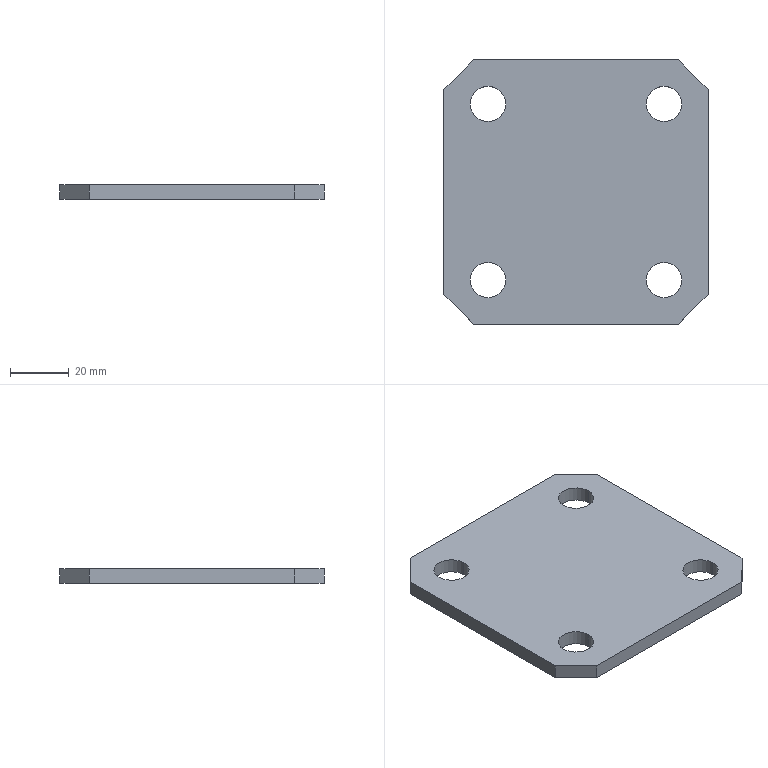Part | STEP file | Floating adjusting plate | 1 solid | 18 faces | box 90 x 90 x 5 mm | volume 37238 mm3 | plane 10 | cylinder 8 | commonest cylinder face diameters 12 x8
STEP:
#1=CARTESIAN_POINT('',(-24.,-30.,5.));
#2=VERTEX_POINT('',#1);
#3=CARTESIAN_POINT('',(-36.,-30.,5.));
#4=VERTEX_POINT('',#3);
#5=CARTESIAN_POINT('',(-30.,-30.,5.));
#6=DIRECTION('',(0.,0.,-1.));
#7=DIRECTION('',(1.,0.,0.));
#8=AXIS2_PLACEMENT_3D('',#5,#6,#7);
#9=CIRCLE('',#8,6.);
#10=EDGE_CURVE('',#2,#4,#9,.T.);
#11=ORIENTED_EDGE('',*,*,#10,.F.);
#12=CARTESIAN_POINT('',(-24.,-30.,0.));
#13=VERTEX_POINT('',#12);
#14=CARTESIAN_POINT('',(-24.,-30.,10.));
#15=DIRECTION('',(0.,0.,-1.));
#16=VECTOR('',#15,1000.);
#17=LINE('',#14,#16);
#18=EDGE_CURVE('',#2,#13,#17,.T.);
#19=ORIENTED_EDGE('',*,*,#18,.T.);
#20=CARTESIAN_POINT('',(-36.,-30.,0.));
#21=VERTEX_POINT('',#20);
#22=CARTESIAN_POINT('',(-30.,-30.,0.));
#23=DIRECTION('',(0.,0.,1.));
#24=DIRECTION('',(1.,0.,0.));
#25=AXIS2_PLACEMENT_3D('',#22,#23,#24);
#26=CIRCLE('',#25,6.);
#27=EDGE_CURVE('',#21,#13,#26,.T.);
#28=ORIENTED_EDGE('',*,*,#27,.F.);
#29=CARTESIAN_POINT('',(-36.,-30.,10.));
#30=DIRECTION('',(0.,0.,-1.));
#31=VECTOR('',#30,1000.);
#32=LINE('',#29,#31);
#33=EDGE_CURVE('',#4,#21,#32,.T.);
#34=ORIENTED_EDGE('',*,*,#33,.F.);
#35=EDGE_LOOP('',(#11,#19,#28,#34));
#36=FACE_OUTER_BOUND('',#35,.T.);
#37=CARTESIAN_POINT('',(-30.,-30.,10.));
#38=DIRECTION('',(0.,0.,-1.));
#39=DIRECTION('',(-1.,0.,0.));
#40=AXIS2_PLACEMENT_3D('',#37,#38,#39);
#41=CYLINDRICAL_SURFACE('',#40,6.);
#42=ADVANCED_FACE('',(#36),#41,.F.);
#43=CARTESIAN_POINT('',(-36.,30.,5.));
#44=VERTEX_POINT('',#43);
#45=CARTESIAN_POINT('',(-24.,30.,5.));
#46=VERTEX_POINT('',#45);
#47=CARTESIAN_POINT('',(-30.,30.,5.));
#48=DIRECTION('',(0.,0.,1.));
#49=DIRECTION('',(1.,0.,0.));
#50=AXIS2_PLACEMENT_3D('',#47,#48,#49);
#51=CIRCLE('',#50,6.);
#52=EDGE_CURVE('',#44,#46,#51,.T.);
#53=ORIENTED_EDGE('',*,*,#52,.T.);
#54=CARTESIAN_POINT('',(-24.,30.,0.));
#55=VERTEX_POINT('',#54);
#56=CARTESIAN_POINT('',(-24.,30.,10.));
#57=DIRECTION('',(0.,0.,-1.));
#58=VECTOR('',#57,1000.);
#59=LINE('',#56,#58);
#60=EDGE_CURVE('',#46,#55,#59,.T.);
#61=ORIENTED_EDGE('',*,*,#60,.T.);
#62=CARTESIAN_POINT('',(-36.,30.,0.));
#63=VERTEX_POINT('',#62);
#64=CARTESIAN_POINT('',(-30.,30.,0.));
#65=DIRECTION('',(0.,0.,-1.));
#66=DIRECTION('',(1.,0.,0.));
#67=AXIS2_PLACEMENT_3D('',#64,#65,#66);
#68=CIRCLE('',#67,6.);
#69=EDGE_CURVE('',#55,#63,#68,.T.);
#70=ORIENTED_EDGE('',*,*,#69,.T.);
#71=CARTESIAN_POINT('',(-36.,30.,10.));
#72=DIRECTION('',(0.,0.,-1.));
#73=VECTOR('',#72,1000.);
#74=LINE('',#71,#73);
#75=EDGE_CURVE('',#44,#63,#74,.T.);
#76=ORIENTED_EDGE('',*,*,#75,.F.);
#77=EDGE_LOOP('',(#53,#61,#70,#76));
#78=FACE_OUTER_BOUND('',#77,.T.);
#79=CARTESIAN_POINT('',(-30.,30.,10.));
#80=DIRECTION('',(0.,0.,-1.));
#81=DIRECTION('',(-1.,0.,0.));
#82=AXIS2_PLACEMENT_3D('',#79,#80,#81);
#83=CYLINDRICAL_SURFACE('',#82,6.);
#84=ADVANCED_FACE('',(#78),#83,.F.);
#85=CARTESIAN_POINT('',(36.,30.,5.));
#86=VERTEX_POINT('',#85);
#87=CARTESIAN_POINT('',(24.,30.,5.));
#88=VERTEX_POINT('',#87);
#89=CARTESIAN_POINT('',(30.,30.,5.));
#90=DIRECTION('',(0.,0.,-1.));
#91=DIRECTION('',(1.,0.,0.));
#92=AXIS2_PLACEMENT_3D('',#89,#90,#91);
#93=CIRCLE('',#92,6.);
#94=EDGE_CURVE('',#86,#88,#93,.T.);
#95=ORIENTED_EDGE('',*,*,#94,.F.);
#96=CARTESIAN_POINT('',(36.,30.,0.));
#97=VERTEX_POINT('',#96);
#98=CARTESIAN_POINT('',(36.,30.,10.));
#99=DIRECTION('',(0.,0.,-1.));
#100=VECTOR('',#99,1000.);
#101=LINE('',#98,#100);
#102=EDGE_CURVE('',#86,#97,#101,.T.);
#103=ORIENTED_EDGE('',*,*,#102,.T.);
#104=CARTESIAN_POINT('',(24.,30.,0.));
#105=VERTEX_POINT('',#104);
#106=CARTESIAN_POINT('',(30.,30.,0.));
#107=DIRECTION('',(0.,0.,1.));
#108=DIRECTION('',(-1.,0.,0.));
#109=AXIS2_PLACEMENT_3D('',#106,#107,#108);
#110=CIRCLE('',#109,6.);
#111=EDGE_CURVE('',#105,#97,#110,.T.);
#112=ORIENTED_EDGE('',*,*,#111,.F.);
#113=CARTESIAN_POINT('',(24.,30.,10.));
#114=DIRECTION('',(0.,0.,-1.));
#115=VECTOR('',#114,1000.);
#116=LINE('',#113,#115);
#117=EDGE_CURVE('',#88,#105,#116,.T.);
#118=ORIENTED_EDGE('',*,*,#117,.F.);
#119=EDGE_LOOP('',(#95,#103,#112,#118));
#120=FACE_OUTER_BOUND('',#119,.T.);
#121=CARTESIAN_POINT('',(30.,30.,10.));
#122=DIRECTION('',(0.,0.,-1.));
#123=DIRECTION('',(-1.,0.,0.));
#124=AXIS2_PLACEMENT_3D('',#121,#122,#123);
#125=CYLINDRICAL_SURFACE('',#124,6.);
#126=ADVANCED_FACE('',(#120),#125,.F.);
#127=CARTESIAN_POINT('',(24.,-30.,5.));
#128=VERTEX_POINT('',#127);
#129=CARTESIAN_POINT('',(36.,-30.,5.));
#130=VERTEX_POINT('',#129);
#131=CARTESIAN_POINT('',(30.,-30.,5.));
#132=DIRECTION('',(0.,0.,1.));
#133=DIRECTION('',(1.,0.,0.));
#134=AXIS2_PLACEMENT_3D('',#131,#132,#133);
#135=CIRCLE('',#134,6.);
#136=EDGE_CURVE('',#128,#130,#135,.T.);
#137=ORIENTED_EDGE('',*,*,#136,.T.);
#138=CARTESIAN_POINT('',(36.,-30.,0.));
#139=VERTEX_POINT('',#138);
#140=CARTESIAN_POINT('',(36.,-30.,10.));
#141=DIRECTION('',(0.,0.,-1.));
#142=VECTOR('',#141,1000.);
#143=LINE('',#140,#142);
#144=EDGE_CURVE('',#130,#139,#143,.T.);
#145=ORIENTED_EDGE('',*,*,#144,.T.);
#146=CARTESIAN_POINT('',(24.,-30.,0.));
#147=VERTEX_POINT('',#146);
#148=CARTESIAN_POINT('',(30.,-30.,0.));
#149=DIRECTION('',(0.,0.,-1.));
#150=DIRECTION('',(-1.,0.,0.));
#151=AXIS2_PLACEMENT_3D('',#148,#149,#150);
#152=CIRCLE('',#151,6.);
#153=EDGE_CURVE('',#139,#147,#152,.T.);
#154=ORIENTED_EDGE('',*,*,#153,.T.);
#155=CARTESIAN_POINT('',(24.,-30.,10.));
#156=DIRECTION('',(0.,0.,-1.));
#157=VECTOR('',#156,1000.);
#158=LINE('',#155,#157);
#159=EDGE_CURVE('',#128,#147,#158,.T.);
#160=ORIENTED_EDGE('',*,*,#159,.F.);
#161=EDGE_LOOP('',(#137,#145,#154,#160));
#162=FACE_OUTER_BOUND('',#161,.T.);
#163=CARTESIAN_POINT('',(30.,-30.,10.));
#164=DIRECTION('',(0.,0.,-1.));
#165=DIRECTION('',(-1.,0.,0.));
#166=AXIS2_PLACEMENT_3D('',#163,#164,#165);
#167=CYLINDRICAL_SURFACE('',#166,6.);
#168=ADVANCED_FACE('',(#162),#167,.F.);
#169=CARTESIAN_POINT('',(45.,-35.,0.));
#170=VERTEX_POINT('',#169);
#171=CARTESIAN_POINT('',(45.,35.,0.));
#172=VERTEX_POINT('',#171);
#173=CARTESIAN_POINT('',(45.,45.,0.));
#174=DIRECTION('',(0.,1.,0.));
#175=VECTOR('',#174,1000.);
#176=LINE('',#173,#175);
#177=EDGE_CURVE('',#170,#172,#176,.T.);
#178=ORIENTED_EDGE('',*,*,#177,.T.);
#179=CARTESIAN_POINT('',(45.,35.,5.));
#180=VERTEX_POINT('',#179);
#181=CARTESIAN_POINT('',(45.,35.,5.));
#182=DIRECTION('',(0.,0.,1.));
#183=VECTOR('',#182,1000.);
#184=LINE('',#181,#183);
#185=EDGE_CURVE('',#172,#180,#184,.T.);
#186=ORIENTED_EDGE('',*,*,#185,.T.);
#187=CARTESIAN_POINT('',(45.,-35.,5.));
#188=VERTEX_POINT('',#187);
#189=CARTESIAN_POINT('',(45.,45.,5.));
#190=DIRECTION('',(0.,1.,0.));
#191=VECTOR('',#190,1000.);
#192=LINE('',#189,#191);
#193=EDGE_CURVE('',#188,#180,#192,.T.);
#194=ORIENTED_EDGE('',*,*,#193,.F.);
#195=CARTESIAN_POINT('',(45.,-35.,5.));
#196=DIRECTION('',(0.,0.,-1.));
#197=VECTOR('',#196,1000.);
#198=LINE('',#195,#197);
#199=EDGE_CURVE('',#188,#170,#198,.T.);
#200=ORIENTED_EDGE('',*,*,#199,.T.);
#201=EDGE_LOOP('',(#178,#186,#194,#200));
#202=FACE_OUTER_BOUND('',#201,.T.);
#203=CARTESIAN_POINT('',(45.,45.,5.));
#204=DIRECTION('',(-1.,0.,0.));
#205=DIRECTION('',(0.,-1.,0.));
#206=AXIS2_PLACEMENT_3D('',#203,#204,#205);
#207=PLANE('',#206);
#208=ADVANCED_FACE('',(#202),#207,.F.);
#209=CARTESIAN_POINT('',(35.,45.,5.));
#210=VERTEX_POINT('',#209);
#211=CARTESIAN_POINT('',(-35.,45.,5.));
#212=VERTEX_POINT('',#211);
#213=CARTESIAN_POINT('',(-45.,45.,5.));
#214=DIRECTION('',(-1.,0.,0.));
#215=VECTOR('',#214,1000.);
#216=LINE('',#213,#215);
#217=EDGE_CURVE('',#210,#212,#216,.T.);
#218=ORIENTED_EDGE('',*,*,#217,.F.);
#219=CARTESIAN_POINT('',(35.,45.,0.));
#220=VERTEX_POINT('',#219);
#221=CARTESIAN_POINT('',(35.,45.,5.));
#222=DIRECTION('',(0.,0.,-1.));
#223=VECTOR('',#222,1000.);
#224=LINE('',#221,#223);
#225=EDGE_CURVE('',#210,#220,#224,.T.);
#226=ORIENTED_EDGE('',*,*,#225,.T.);
#227=CARTESIAN_POINT('',(-35.,45.,0.));
#228=VERTEX_POINT('',#227);
#229=CARTESIAN_POINT('',(-45.,45.,0.));
#230=DIRECTION('',(-1.,0.,0.));
#231=VECTOR('',#230,1000.);
#232=LINE('',#229,#231);
#233=EDGE_CURVE('',#220,#228,#232,.T.);
#234=ORIENTED_EDGE('',*,*,#233,.T.);
#235=CARTESIAN_POINT('',(-35.,45.,5.));
#236=DIRECTION('',(0.,0.,1.));
#237=VECTOR('',#236,1000.);
#238=LINE('',#235,#237);
#239=EDGE_CURVE('',#228,#212,#238,.T.);
#240=ORIENTED_EDGE('',*,*,#239,.T.);
#241=EDGE_LOOP('',(#218,#226,#234,#240));
#242=FACE_OUTER_BOUND('',#241,.T.);
#243=CARTESIAN_POINT('',(-45.,45.,5.));
#244=DIRECTION('',(0.,-1.,0.));
#245=DIRECTION('',(0.,0.,-1.));
#246=AXIS2_PLACEMENT_3D('',#243,#244,#245);
#247=PLANE('',#246);
#248=ADVANCED_FACE('',(#242),#247,.F.);
#249=CARTESIAN_POINT('',(-45.,35.,5.));
#250=VERTEX_POINT('',#249);
#251=CARTESIAN_POINT('',(-45.,-35.,5.));
#252=VERTEX_POINT('',#251);
#253=CARTESIAN_POINT('',(-45.,45.,5.));
#254=DIRECTION('',(0.,-1.,0.));
#255=VECTOR('',#254,1000.);
#256=LINE('',#253,#255);
#257=EDGE_CURVE('',#250,#252,#256,.T.);
#258=ORIENTED_EDGE('',*,*,#257,.F.);
#259=CARTESIAN_POINT('',(-45.,35.,0.));
#260=VERTEX_POINT('',#259);
#261=CARTESIAN_POINT('',(-45.,35.,5.));
#262=DIRECTION('',(0.,0.,-1.));
#263=VECTOR('',#262,1000.);
#264=LINE('',#261,#263);
#265=EDGE_CURVE('',#250,#260,#264,.T.);
#266=ORIENTED_EDGE('',*,*,#265,.T.);
#267=CARTESIAN_POINT('',(-45.,-35.,0.));
#268=VERTEX_POINT('',#267);
#269=CARTESIAN_POINT('',(-45.,45.,0.));
#270=DIRECTION('',(0.,-1.,0.));
#271=VECTOR('',#270,1000.);
#272=LINE('',#269,#271);
#273=EDGE_CURVE('',#260,#268,#272,.T.);
#274=ORIENTED_EDGE('',*,*,#273,.T.);
#275=CARTESIAN_POINT('',(-45.,-35.,5.));
#276=DIRECTION('',(0.,0.,1.));
#277=VECTOR('',#276,1000.);
#278=LINE('',#275,#277);
#279=EDGE_CURVE('',#268,#252,#278,.T.);
#280=ORIENTED_EDGE('',*,*,#279,.T.);
#281=EDGE_LOOP('',(#258,#266,#274,#280));
#282=FACE_OUTER_BOUND('',#281,.T.);
#283=CARTESIAN_POINT('',(-45.,45.,5.));
#284=DIRECTION('',(1.,0.,0.));
#285=DIRECTION('',(0.,1.,0.));
#286=AXIS2_PLACEMENT_3D('',#283,#284,#285);
#287=PLANE('',#286);
#288=ADVANCED_FACE('',(#282),#287,.F.);
#289=CARTESIAN_POINT('',(-35.,-45.,5.));
#290=VERTEX_POINT('',#289);
#291=CARTESIAN_POINT('',(35.,-45.,5.));
#292=VERTEX_POINT('',#291);
#293=CARTESIAN_POINT('',(-45.,-45.,5.));
#294=DIRECTION('',(1.,0.,0.));
#295=VECTOR('',#294,1000.);
#296=LINE('',#293,#295);
#297=EDGE_CURVE('',#290,#292,#296,.T.);
#298=ORIENTED_EDGE('',*,*,#297,.F.);
#299=CARTESIAN_POINT('',(-35.,-45.,0.));
#300=VERTEX_POINT('',#299);
#301=CARTESIAN_POINT('',(-35.,-45.,5.));
#302=DIRECTION('',(0.,0.,-1.));
#303=VECTOR('',#302,1000.);
#304=LINE('',#301,#303);
#305=EDGE_CURVE('',#290,#300,#304,.T.);
#306=ORIENTED_EDGE('',*,*,#305,.T.);
#307=CARTESIAN_POINT('',(35.,-45.,0.));
#308=VERTEX_POINT('',#307);
#309=CARTESIAN_POINT('',(-45.,-45.,0.));
#310=DIRECTION('',(1.,0.,0.));
#311=VECTOR('',#310,1000.);
#312=LINE('',#309,#311);
#313=EDGE_CURVE('',#300,#308,#312,.T.);
#314=ORIENTED_EDGE('',*,*,#313,.T.);
#315=CARTESIAN_POINT('',(35.,-45.,5.));
#316=DIRECTION('',(0.,0.,1.));
#317=VECTOR('',#316,1000.);
#318=LINE('',#315,#317);
#319=EDGE_CURVE('',#308,#292,#318,.T.);
#320=ORIENTED_EDGE('',*,*,#319,.T.);
#321=EDGE_LOOP('',(#298,#306,#314,#320));
#322=FACE_OUTER_BOUND('',#321,.T.);
#323=CARTESIAN_POINT('',(-45.,-45.,5.));
#324=DIRECTION('',(0.,1.,0.));
#325=DIRECTION('',(0.,0.,1.));
#326=AXIS2_PLACEMENT_3D('',#323,#324,#325);
#327=PLANE('',#326);
#328=ADVANCED_FACE('',(#322),#327,.F.);
#329=CARTESIAN_POINT('',(-30.,-30.,5.));
#330=DIRECTION('',(0.,0.,-1.));
#331=DIRECTION('',(1.,0.,0.));
#332=AXIS2_PLACEMENT_3D('',#329,#330,#331);
#333=CIRCLE('',#332,6.);
#334=EDGE_CURVE('',#4,#2,#333,.T.);
#335=ORIENTED_EDGE('',*,*,#334,.T.);
#336=ORIENTED_EDGE('',*,*,#10,.T.);
#337=EDGE_LOOP('',(#335,#336));
#338=FACE_BOUND('',#337,.T.);
#339=ORIENTED_EDGE('',*,*,#52,.F.);
#340=CARTESIAN_POINT('',(-30.,30.,5.));
#341=DIRECTION('',(0.,0.,1.));
#342=DIRECTION('',(1.,0.,0.));
#343=AXIS2_PLACEMENT_3D('',#340,#341,#342);
#344=CIRCLE('',#343,6.);
#345=EDGE_CURVE('',#46,#44,#344,.T.);
#346=ORIENTED_EDGE('',*,*,#345,.F.);
#347=EDGE_LOOP('',(#339,#346));
#348=FACE_BOUND('',#347,.T.);
#349=CARTESIAN_POINT('',(30.,30.,5.));
#350=DIRECTION('',(0.,0.,-1.));
#351=DIRECTION('',(1.,0.,0.));
#352=AXIS2_PLACEMENT_3D('',#349,#350,#351);
#353=CIRCLE('',#352,6.);
#354=EDGE_CURVE('',#88,#86,#353,.T.);
#355=ORIENTED_EDGE('',*,*,#354,.T.);
#356=ORIENTED_EDGE('',*,*,#94,.T.);
#357=EDGE_LOOP('',(#355,#356));
#358=FACE_BOUND('',#357,.T.);
#359=ORIENTED_EDGE('',*,*,#136,.F.);
#360=CARTESIAN_POINT('',(30.,-30.,5.));
#361=DIRECTION('',(0.,0.,1.));
#362=DIRECTION('',(1.,0.,0.));
#363=AXIS2_PLACEMENT_3D('',#360,#361,#362);
#364=CIRCLE('',#363,6.);
#365=EDGE_CURVE('',#130,#128,#364,.T.);
#366=ORIENTED_EDGE('',*,*,#365,.F.);
#367=EDGE_LOOP('',(#359,#366));
#368=FACE_BOUND('',#367,.T.);
#369=ORIENTED_EDGE('',*,*,#193,.T.);
#370=CARTESIAN_POINT('',(40.,40.,5.));
#371=DIRECTION('',(-0.7071,0.7071,0.));
#372=VECTOR('',#371,1000.);
#373=LINE('',#370,#372);
#374=EDGE_CURVE('',#180,#210,#373,.T.);
#375=ORIENTED_EDGE('',*,*,#374,.T.);
#376=ORIENTED_EDGE('',*,*,#217,.T.);
#377=CARTESIAN_POINT('',(-40.,40.,5.));
#378=DIRECTION('',(-0.7071,-0.7071,0.));
#379=VECTOR('',#378,1000.);
#380=LINE('',#377,#379);
#381=EDGE_CURVE('',#212,#250,#380,.T.);
#382=ORIENTED_EDGE('',*,*,#381,.T.);
#383=ORIENTED_EDGE('',*,*,#257,.T.);
#384=CARTESIAN_POINT('',(-40.,-40.,5.));
#385=DIRECTION('',(0.7071,-0.7071,0.));
#386=VECTOR('',#385,1000.);
#387=LINE('',#384,#386);
#388=EDGE_CURVE('',#252,#290,#387,.T.);
#389=ORIENTED_EDGE('',*,*,#388,.T.);
#390=ORIENTED_EDGE('',*,*,#297,.T.);
#391=CARTESIAN_POINT('',(40.,-40.,5.));
#392=DIRECTION('',(0.7071,0.7071,0.));
#393=VECTOR('',#392,1000.);
#394=LINE('',#391,#393);
#395=EDGE_CURVE('',#292,#188,#394,.T.);
#396=ORIENTED_EDGE('',*,*,#395,.T.);
#397=EDGE_LOOP('',(#369,#375,#376,#382,#383,#389,#390,#396));
#398=FACE_OUTER_BOUND('',#397,.T.);
#399=CARTESIAN_POINT('',(0.,0.,5.));
#400=DIRECTION('',(0.,0.,1.));
#401=DIRECTION('',(1.,0.,0.));
#402=AXIS2_PLACEMENT_3D('',#399,#400,#401);
#403=PLANE('',#402);
#404=ADVANCED_FACE('',(#338,#348,#358,#368,#398),#403,.T.);
#405=ORIENTED_EDGE('',*,*,#27,.T.);
#406=CARTESIAN_POINT('',(-30.,-30.,0.));
#407=DIRECTION('',(0.,0.,1.));
#408=DIRECTION('',(1.,0.,0.));
#409=AXIS2_PLACEMENT_3D('',#406,#407,#408);
#410=CIRCLE('',#409,6.);
#411=EDGE_CURVE('',#13,#21,#410,.T.);
#412=ORIENTED_EDGE('',*,*,#411,.T.);
#413=EDGE_LOOP('',(#405,#412));
#414=FACE_BOUND('',#413,.T.);
#415=CARTESIAN_POINT('',(-30.,30.,0.));
#416=DIRECTION('',(0.,0.,-1.));
#417=DIRECTION('',(1.,0.,0.));
#418=AXIS2_PLACEMENT_3D('',#415,#416,#417);
#419=CIRCLE('',#418,6.);
#420=EDGE_CURVE('',#63,#55,#419,.T.);
#421=ORIENTED_EDGE('',*,*,#420,.F.);
#422=ORIENTED_EDGE('',*,*,#69,.F.);
#423=EDGE_LOOP('',(#421,#422));
#424=FACE_BOUND('',#423,.T.);
#425=ORIENTED_EDGE('',*,*,#111,.T.);
#426=CARTESIAN_POINT('',(30.,30.,0.));
#427=DIRECTION('',(0.,0.,1.));
#428=DIRECTION('',(-1.,0.,0.));
#429=AXIS2_PLACEMENT_3D('',#426,#427,#428);
#430=CIRCLE('',#429,6.);
#431=EDGE_CURVE('',#97,#105,#430,.T.);
#432=ORIENTED_EDGE('',*,*,#431,.T.);
#433=EDGE_LOOP('',(#425,#432));
#434=FACE_BOUND('',#433,.T.);
#435=CARTESIAN_POINT('',(30.,-30.,0.));
#436=DIRECTION('',(0.,0.,-1.));
#437=DIRECTION('',(-1.,0.,0.));
#438=AXIS2_PLACEMENT_3D('',#435,#436,#437);
#439=CIRCLE('',#438,6.);
#440=EDGE_CURVE('',#147,#139,#439,.T.);
#441=ORIENTED_EDGE('',*,*,#440,.F.);
#442=ORIENTED_EDGE('',*,*,#153,.F.);
#443=EDGE_LOOP('',(#441,#442));
#444=FACE_BOUND('',#443,.T.);
#445=ORIENTED_EDGE('',*,*,#233,.F.);
#446=CARTESIAN_POINT('',(35.,45.,0.));
#447=DIRECTION('',(0.7071,-0.7071,0.));
#448=VECTOR('',#447,1000.);
#449=LINE('',#446,#448);
#450=EDGE_CURVE('',#220,#172,#449,.T.);
#451=ORIENTED_EDGE('',*,*,#450,.T.);
#452=ORIENTED_EDGE('',*,*,#177,.F.);
#453=CARTESIAN_POINT('',(45.,-35.,0.));
#454=DIRECTION('',(-0.7071,-0.7071,0.));
#455=VECTOR('',#454,1000.);
#456=LINE('',#453,#455);
#457=EDGE_CURVE('',#170,#308,#456,.T.);
#458=ORIENTED_EDGE('',*,*,#457,.T.);
#459=ORIENTED_EDGE('',*,*,#313,.F.);
#460=CARTESIAN_POINT('',(-35.,-45.,0.));
#461=DIRECTION('',(-0.7071,0.7071,0.));
#462=VECTOR('',#461,1000.);
#463=LINE('',#460,#462);
#464=EDGE_CURVE('',#300,#268,#463,.T.);
#465=ORIENTED_EDGE('',*,*,#464,.T.);
#466=ORIENTED_EDGE('',*,*,#273,.F.);
#467=CARTESIAN_POINT('',(-45.,35.,0.));
#468=DIRECTION('',(0.7071,0.7071,0.));
#469=VECTOR('',#468,1000.);
#470=LINE('',#467,#469);
#471=EDGE_CURVE('',#260,#228,#470,.T.);
#472=ORIENTED_EDGE('',*,*,#471,.T.);
#473=EDGE_LOOP('',(#445,#451,#452,#458,#459,#465,#466,#472));
#474=FACE_OUTER_BOUND('',#473,.T.);
#475=CARTESIAN_POINT('',(0.,0.,0.));
#476=DIRECTION('',(0.,0.,1.));
#477=DIRECTION('',(1.,0.,0.));
#478=AXIS2_PLACEMENT_3D('',#475,#476,#477);
#479=PLANE('',#478);
#480=ADVANCED_FACE('',(#414,#424,#434,#444,#474),#479,.F.);
#481=ORIENTED_EDGE('',*,*,#144,.F.);
#482=ORIENTED_EDGE('',*,*,#365,.T.);
#483=ORIENTED_EDGE('',*,*,#159,.T.);
#484=ORIENTED_EDGE('',*,*,#440,.T.);
#485=EDGE_LOOP('',(#481,#482,#483,#484));
#486=FACE_OUTER_BOUND('',#485,.T.);
#487=CARTESIAN_POINT('',(30.,-30.,10.));
#488=DIRECTION('',(0.,0.,-1.));
#489=DIRECTION('',(-1.,0.,0.));
#490=AXIS2_PLACEMENT_3D('',#487,#488,#489);
#491=CYLINDRICAL_SURFACE('',#490,6.);
#492=ADVANCED_FACE('',(#486),#491,.F.);
#493=ORIENTED_EDGE('',*,*,#102,.F.);
#494=ORIENTED_EDGE('',*,*,#354,.F.);
#495=ORIENTED_EDGE('',*,*,#117,.T.);
#496=ORIENTED_EDGE('',*,*,#431,.F.);
#497=EDGE_LOOP('',(#493,#494,#495,#496));
#498=FACE_OUTER_BOUND('',#497,.T.);
#499=CARTESIAN_POINT('',(30.,30.,10.));
#500=DIRECTION('',(0.,0.,-1.));
#501=DIRECTION('',(-1.,0.,0.));
#502=AXIS2_PLACEMENT_3D('',#499,#500,#501);
#503=CYLINDRICAL_SURFACE('',#502,6.);
#504=ADVANCED_FACE('',(#498),#503,.F.);
#505=ORIENTED_EDGE('',*,*,#60,.F.);
#506=ORIENTED_EDGE('',*,*,#345,.T.);
#507=ORIENTED_EDGE('',*,*,#75,.T.);
#508=ORIENTED_EDGE('',*,*,#420,.T.);
#509=EDGE_LOOP('',(#505,#506,#507,#508));
#510=FACE_OUTER_BOUND('',#509,.T.);
#511=CARTESIAN_POINT('',(-30.,30.,10.));
#512=DIRECTION('',(0.,0.,-1.));
#513=DIRECTION('',(-1.,0.,0.));
#514=AXIS2_PLACEMENT_3D('',#511,#512,#513);
#515=CYLINDRICAL_SURFACE('',#514,6.);
#516=ADVANCED_FACE('',(#510),#515,.F.);
#517=ORIENTED_EDGE('',*,*,#18,.F.);
#518=ORIENTED_EDGE('',*,*,#334,.F.);
#519=ORIENTED_EDGE('',*,*,#33,.T.);
#520=ORIENTED_EDGE('',*,*,#411,.F.);
#521=EDGE_LOOP('',(#517,#518,#519,#520));
#522=FACE_OUTER_BOUND('',#521,.T.);
#523=CARTESIAN_POINT('',(-30.,-30.,10.));
#524=DIRECTION('',(0.,0.,-1.));
#525=DIRECTION('',(-1.,0.,0.));
#526=AXIS2_PLACEMENT_3D('',#523,#524,#525);
#527=CYLINDRICAL_SURFACE('',#526,6.);
#528=ADVANCED_FACE('',(#522),#527,.F.);
#529=ORIENTED_EDGE('',*,*,#374,.F.);
#530=ORIENTED_EDGE('',*,*,#185,.F.);
#531=ORIENTED_EDGE('',*,*,#450,.F.);
#532=ORIENTED_EDGE('',*,*,#225,.F.);
#533=EDGE_LOOP('',(#529,#530,#531,#532));
#534=FACE_OUTER_BOUND('',#533,.T.);
#535=CARTESIAN_POINT('',(35.,45.,5.));
#536=DIRECTION('',(-0.7071,-0.7071,0.));
#537=DIRECTION('',(0.,0.,-1.));
#538=AXIS2_PLACEMENT_3D('',#535,#536,#537);
#539=PLANE('',#538);
#540=ADVANCED_FACE('',(#534),#539,.F.);
#541=ORIENTED_EDGE('',*,*,#381,.F.);
#542=ORIENTED_EDGE('',*,*,#239,.F.);
#543=ORIENTED_EDGE('',*,*,#471,.F.);
#544=ORIENTED_EDGE('',*,*,#265,.F.);
#545=EDGE_LOOP('',(#541,#542,#543,#544));
#546=FACE_OUTER_BOUND('',#545,.T.);
#547=CARTESIAN_POINT('',(-45.,35.,5.));
#548=DIRECTION('',(0.7071,-0.7071,0.));
#549=DIRECTION('',(0.,0.,-1.));
#550=AXIS2_PLACEMENT_3D('',#547,#548,#549);
#551=PLANE('',#550);
#552=ADVANCED_FACE('',(#546),#551,.F.);
#553=ORIENTED_EDGE('',*,*,#388,.F.);
#554=ORIENTED_EDGE('',*,*,#279,.F.);
#555=ORIENTED_EDGE('',*,*,#464,.F.);
#556=ORIENTED_EDGE('',*,*,#305,.F.);
#557=EDGE_LOOP('',(#553,#554,#555,#556));
#558=FACE_OUTER_BOUND('',#557,.T.);
#559=CARTESIAN_POINT('',(-35.,-45.,5.));
#560=DIRECTION('',(0.7071,0.7071,0.));
#561=DIRECTION('',(0.,0.,-1.));
#562=AXIS2_PLACEMENT_3D('',#559,#560,#561);
#563=PLANE('',#562);
#564=ADVANCED_FACE('',(#558),#563,.F.);
#565=ORIENTED_EDGE('',*,*,#395,.F.);
#566=ORIENTED_EDGE('',*,*,#319,.F.);
#567=ORIENTED_EDGE('',*,*,#457,.F.);
#568=ORIENTED_EDGE('',*,*,#199,.F.);
#569=EDGE_LOOP('',(#565,#566,#567,#568));
#570=FACE_OUTER_BOUND('',#569,.T.);
#571=CARTESIAN_POINT('',(45.,-35.,5.));
#572=DIRECTION('',(-0.7071,0.7071,0.));
#573=DIRECTION('',(0.,0.,-1.));
#574=AXIS2_PLACEMENT_3D('',#571,#572,#573);
#575=PLANE('',#574);
#576=ADVANCED_FACE('',(#570),#575,.F.);
#577=CLOSED_SHELL('',(#42,#84,#126,#168,#208,#248,#288,#328,#404,#480,#492,#504,#516,#528,#540,#552,#564,#576));
#578=MANIFOLD_SOLID_BREP('',#577);
#579=CARTESIAN_POINT('',(0.,0.,0.));
#580=DIRECTION('',(0.,0.,1.));
#581=DIRECTION('',(1.,0.,0.));
#582=AXIS2_PLACEMENT_3D('',#579,#580,#581);
#583=(LENGTH_UNIT()NAMED_UNIT(*)SI_UNIT(.MILLI.,.METRE.));
#584=UNCERTAINTY_MEASURE_WITH_UNIT(LENGTH_MEASURE(0.00001),#583,'','');
#585=(NAMED_UNIT(*)PLANE_ANGLE_UNIT()SI_UNIT($,.RADIAN.));
#586=(NAMED_UNIT(*)SI_UNIT($,.STERADIAN.)SOLID_ANGLE_UNIT());
#587=(GEOMETRIC_REPRESENTATION_CONTEXT(3)GLOBAL_UNCERTAINTY_ASSIGNED_CONTEXT((#584))GLOBAL_UNIT_ASSIGNED_CONTEXT((#583,#585,#586))REPRESENTATION_CONTEXT('',''));
#588=ADVANCED_BREP_SHAPE_REPRESENTATION('',(#578,#582),#587);